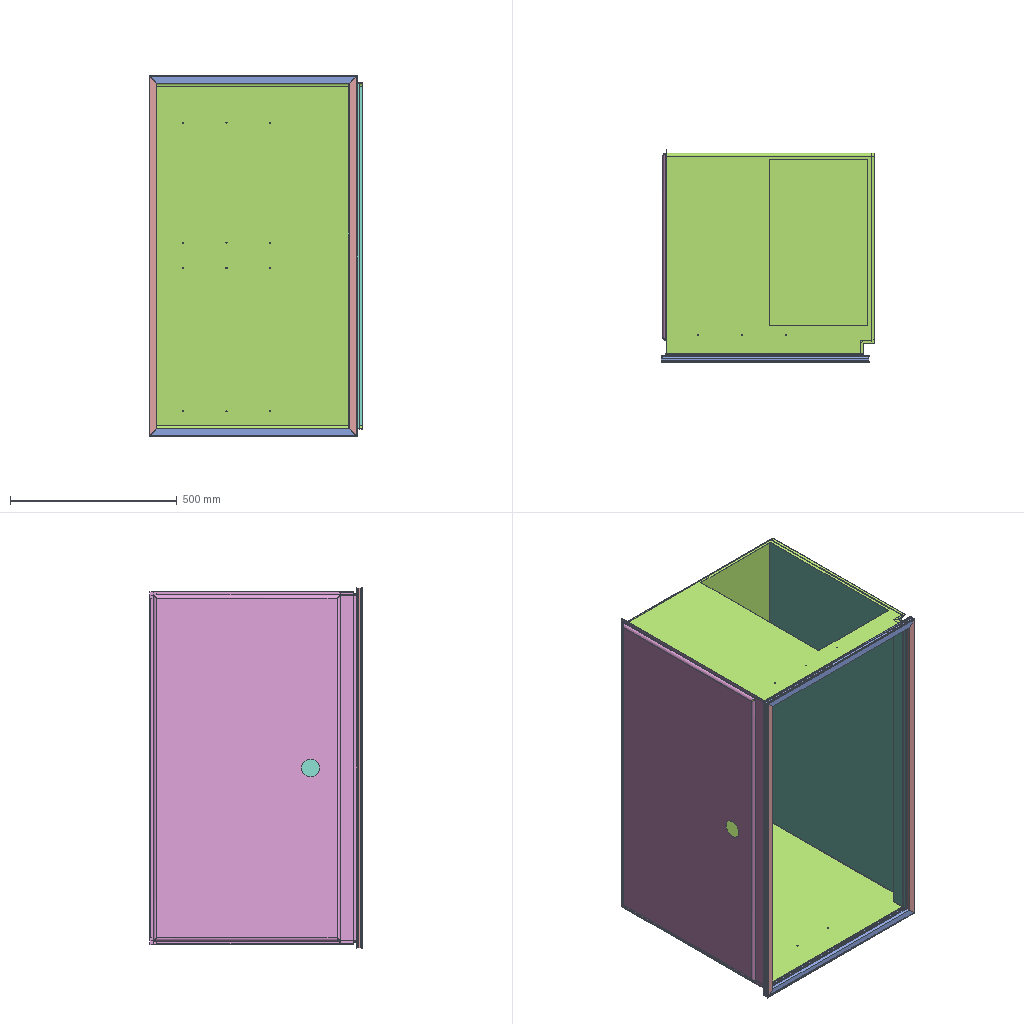Assembly | SolidWorks | 6 different items | 8 placed | box 641 x 636 x 1081 mm
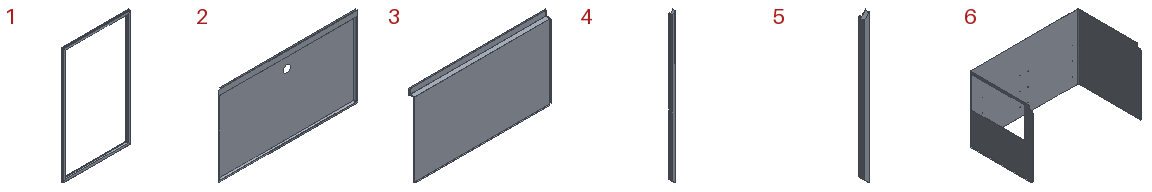Parts list (item | name | quantity | parent item | size | volume | features):
1 | (subassembly) | x1 | - | 624 x 25 x 1081 mm | 1098495 mm3 | -
2 | - | x1 | - | 1058 x 10.6 x 620.2 mm | 404169 mm3 | features EdgeFlange 4, SMWeldBead 2, FlatPattern 1, ICE 1, SMBaseFlange 1, SheetMetal 1
3 | - | x1 | - | 1037 x 44.4 x 608.8 mm | 412914 mm3 | features EdgeFlange 5, Fillet 1, FlatPattern 1, SMBaseFlange 1, SheetMetal 1
4 | - | x2 | in 1 | 22 x 25 x 1081 mm | 350449 mm3 | features ICE 2, Extrusion 1
5 | - | x2 | in 1 | 22 x 25 x 624 mm | 198799 mm3 | features Extrusion 1, ICE 1
6 | - | x1 | - | 1056 x 619.4 x 625.6 mm | 765945 mm3 | features ICE 6, EdgeFlange 3, FlatPattern 1, SMBaseFlange 1, SheetMetal 1, UnFold 1
Mates (type | each side: item.copy, entity, surface, feature):
In the top assembly
Coincident | 5.1 face plane Extrude1 | 6.1 face plane Edge-Flange2
Coincident | 5.1 face plane Extrude1 | 6.1 face plane Edge-Flange3
Coincident | 4.1 face plane Extrude1 | 3.1 face plane Edge-Flange4
Coincident | 6.1 face plane Base-Flange1 | 3.1 face plane Edge-Flange1 | 2 times
Coincident | 4.2 face plane Extrude1 | 2.1 face plane Edge-Flange4
Coincident | 6.1 face plane Edge-Flange1 | 2.1 face plane Edge-Flange3 | 2 times
In subassembly 1
Coincident | 4.3 face plane Extrude5 | 5.2 face plane Extrude2
Coincident | 4.3 face plane Extrude1 | 5.2 face plane Extrude1
Coincident | 4.3 edge | 5.2 edge
Coincident | 4.3 face plane Extrude4 | 5.3 face plane Extrude2
Coincident | 4.3 face plane Extrude1 | 5.3 face plane Extrude1
Coincident | 4.3 edge | 5.3 edge
Coincident | 5.3 face plane Extrude2 | 4.4 face plane Extrude5
Coincident | 5.3 face plane Extrude1 | 4.4 face plane Extrude1
Coincident | 5.3 edge | 4.4 edge